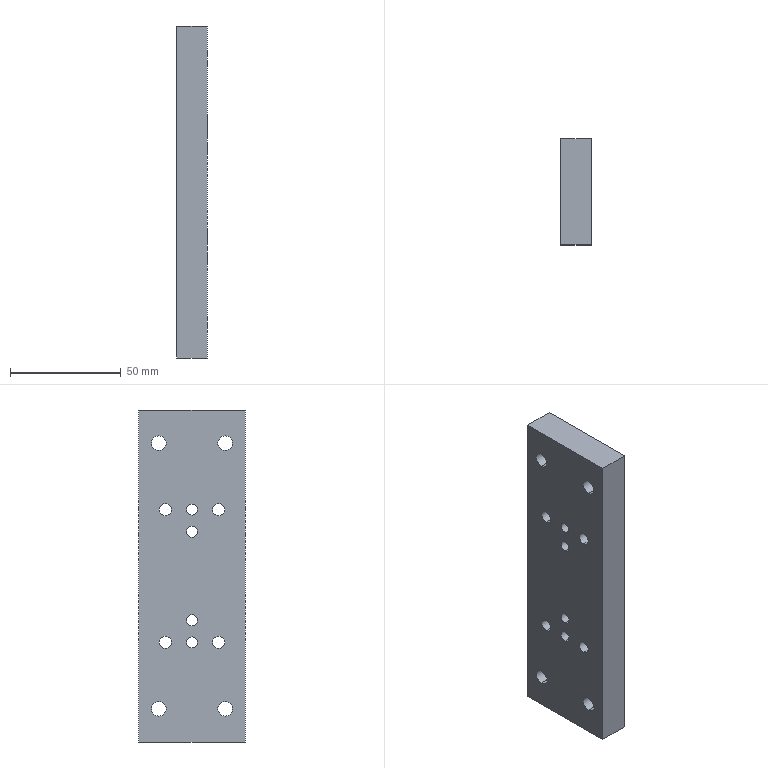Part | STEP file | PN_0064 fixing plate | 1 solid | 42 faces | box 14 x 48 x 150 mm | volume 95205 mm3 | cylinder 32 | plane 10 | commonest cylinder face diameters 5 x8 5.5 x8 6.6 x8 10 x8